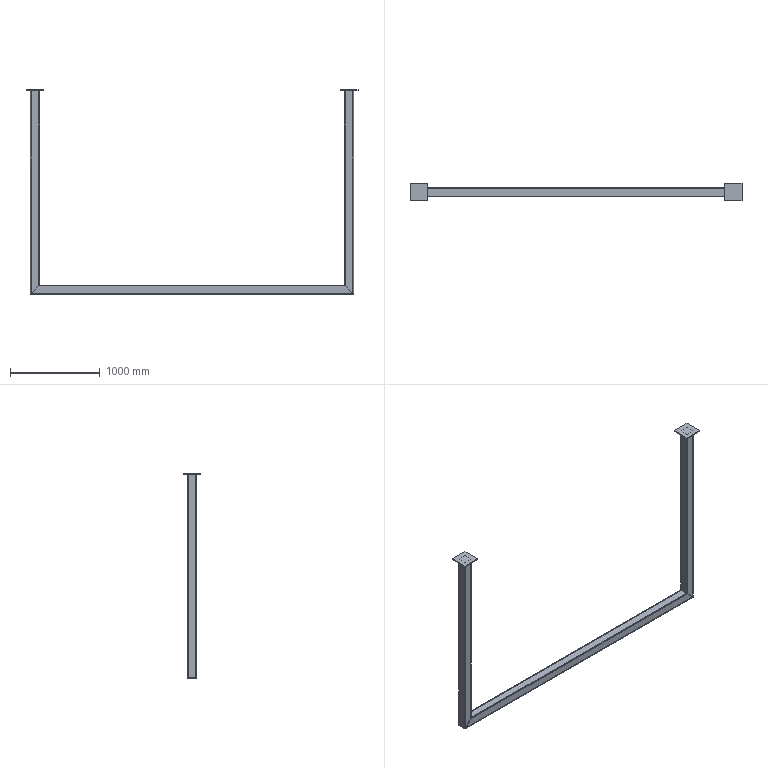Part | STEP file | Bracket_Default<Machined> | 5 solids | 66 faces | box 3700 x 200 x 2275 mm | volume 12653736 mm3 | plane 42 | cylinder 24 | commonest cylinder face diameters 8 x12 16 x12